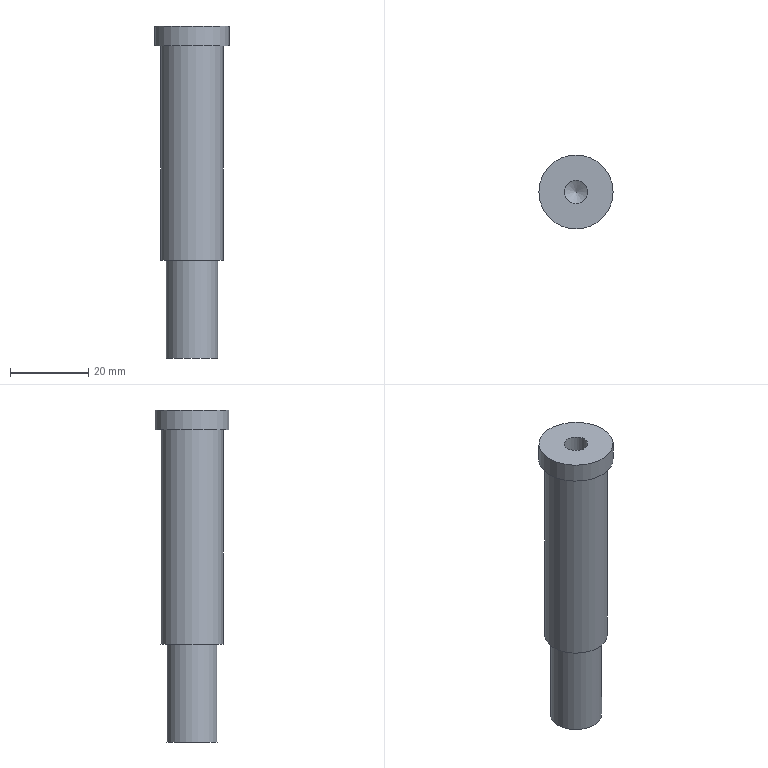Part | NX | features solid 2 | 1 solid | 9 faces | box 19 x 19 x 85 mm | volume 15462 mm3 | cylinder 4 | plane 4 | cone 1 | commonest cylinder face diameters 6 x1 13.1 x1 16 x1 19 x1
STEP:
#1=CARTESIAN_POINT('',(315.095,40.004,20.));
#2=VERTEX_POINT('',#1);
#3=CARTESIAN_POINT('',(307.095,40.004,20.));
#4=DIRECTION('',(0.,0.,1.));
#5=DIRECTION('',(1.,0.,0.));
#6=AXIS2_PLACEMENT_3D('',#3,#4,#5);
#7=CIRCLE('',#6,8.);
#8=EDGE_CURVE('',#2,#2,#7,.T.);
#9=ORIENTED_EDGE('',*,*,#8,.T.);
#10=EDGE_LOOP('',(#9));
#11=FACE_BOUND('',#10,.T.);
#12=CARTESIAN_POINT('',(315.095,40.004,75.));
#13=VERTEX_POINT('',#12);
#14=CARTESIAN_POINT('',(307.095,40.004,75.));
#15=DIRECTION('',(0.,0.,1.));
#16=DIRECTION('',(1.,0.,0.));
#17=AXIS2_PLACEMENT_3D('',#14,#15,#16);
#18=CIRCLE('',#17,8.);
#19=EDGE_CURVE('',#13,#13,#18,.T.);
#20=ORIENTED_EDGE('',*,*,#19,.F.);
#21=EDGE_LOOP('',(#20));
#22=FACE_BOUND('',#21,.T.);
#23=CARTESIAN_POINT('',(307.095,40.004,75.));
#24=DIRECTION('',(0.,0.,-1.));
#25=DIRECTION('',(-1.,0.,0.));
#26=AXIS2_PLACEMENT_3D('',#23,#24,#25);
#27=CYLINDRICAL_SURFACE('',#26,8.);
#28=ADVANCED_FACE('',(#11,#22),#27,.T.);
#29=CARTESIAN_POINT('',(313.645,40.004,20.));
#30=VERTEX_POINT('',#29);
#31=CARTESIAN_POINT('',(307.095,40.004,20.));
#32=DIRECTION('',(0.,0.,1.));
#33=DIRECTION('',(1.,0.,0.));
#34=AXIS2_PLACEMENT_3D('',#31,#32,#33);
#35=CIRCLE('',#34,6.55);
#36=EDGE_CURVE('',#30,#30,#35,.T.);
#37=ORIENTED_EDGE('',*,*,#36,.T.);
#38=EDGE_LOOP('',(#37));
#39=FACE_BOUND('',#38,.T.);
#40=ORIENTED_EDGE('',*,*,#8,.F.);
#41=EDGE_LOOP('',(#40));
#42=FACE_BOUND('',#41,.T.);
#43=CARTESIAN_POINT('',(307.095,40.004,20.));
#44=DIRECTION('',(0.,0.,1.));
#45=DIRECTION('',(1.,0.,0.));
#46=AXIS2_PLACEMENT_3D('',#43,#44,#45);
#47=PLANE('',#46);
#48=ADVANCED_FACE('',(#39,#42),#47,.F.);
#49=CARTESIAN_POINT('',(316.595,40.004,75.));
#50=VERTEX_POINT('',#49);
#51=CARTESIAN_POINT('',(307.095,40.004,75.));
#52=DIRECTION('',(0.,0.,1.));
#53=DIRECTION('',(1.,0.,0.));
#54=AXIS2_PLACEMENT_3D('',#51,#52,#53);
#55=CIRCLE('',#54,9.5);
#56=EDGE_CURVE('',#50,#50,#55,.T.);
#57=ORIENTED_EDGE('',*,*,#56,.F.);
#58=EDGE_LOOP('',(#57));
#59=FACE_BOUND('',#58,.T.);
#60=ORIENTED_EDGE('',*,*,#19,.T.);
#61=EDGE_LOOP('',(#60));
#62=FACE_BOUND('',#61,.T.);
#63=CARTESIAN_POINT('',(307.095,40.004,75.));
#64=DIRECTION('',(0.,0.,1.));
#65=DIRECTION('',(1.,0.,0.));
#66=AXIS2_PLACEMENT_3D('',#63,#64,#65);
#67=PLANE('',#66);
#68=ADVANCED_FACE('',(#59,#62),#67,.F.);
#69=ORIENTED_EDGE('',*,*,#56,.T.);
#70=EDGE_LOOP('',(#69));
#71=FACE_BOUND('',#70,.T.);
#72=CARTESIAN_POINT('',(316.595,40.004,80.));
#73=VERTEX_POINT('',#72);
#74=CARTESIAN_POINT('',(307.095,40.004,80.));
#75=DIRECTION('',(0.,0.,1.));
#76=DIRECTION('',(1.,0.,0.));
#77=AXIS2_PLACEMENT_3D('',#74,#75,#76);
#78=CIRCLE('',#77,9.5);
#79=EDGE_CURVE('',#73,#73,#78,.T.);
#80=ORIENTED_EDGE('',*,*,#79,.F.);
#81=EDGE_LOOP('',(#80));
#82=FACE_BOUND('',#81,.T.);
#83=CARTESIAN_POINT('',(307.095,40.004,70.));
#84=DIRECTION('',(0.,0.,1.));
#85=DIRECTION('',(1.,0.,0.));
#86=AXIS2_PLACEMENT_3D('',#83,#84,#85);
#87=CYLINDRICAL_SURFACE('',#86,9.5);
#88=ADVANCED_FACE('',(#71,#82),#87,.T.);
#89=CARTESIAN_POINT('',(304.095,40.004,80.));
#90=VERTEX_POINT('',#89);
#91=CARTESIAN_POINT('',(307.095,40.004,80.));
#92=DIRECTION('',(0.,0.,-1.));
#93=DIRECTION('',(-1.,0.,0.));
#94=AXIS2_PLACEMENT_3D('',#91,#92,#93);
#95=CIRCLE('',#94,3.);
#96=EDGE_CURVE('',#90,#90,#95,.T.);
#97=ORIENTED_EDGE('',*,*,#96,.T.);
#98=EDGE_LOOP('',(#97));
#99=FACE_BOUND('',#98,.T.);
#100=ORIENTED_EDGE('',*,*,#79,.T.);
#101=EDGE_LOOP('',(#100));
#102=FACE_BOUND('',#101,.T.);
#103=CARTESIAN_POINT('',(307.095,40.004,80.));
#104=DIRECTION('',(0.,0.,1.));
#105=DIRECTION('',(1.,0.,0.));
#106=AXIS2_PLACEMENT_3D('',#103,#104,#105);
#107=PLANE('',#106);
#108=ADVANCED_FACE('',(#99,#102),#107,.T.);
#109=CARTESIAN_POINT('',(313.645,40.004,-5.));
#110=VERTEX_POINT('',#109);
#111=CARTESIAN_POINT('',(307.095,40.004,-5.));
#112=DIRECTION('',(0.,0.,1.));
#113=DIRECTION('',(1.,0.,0.));
#114=AXIS2_PLACEMENT_3D('',#111,#112,#113);
#115=CIRCLE('',#114,6.55);
#116=EDGE_CURVE('',#110,#110,#115,.T.);
#117=ORIENTED_EDGE('',*,*,#116,.T.);
#118=EDGE_LOOP('',(#117));
#119=FACE_BOUND('',#118,.T.);
#120=ORIENTED_EDGE('',*,*,#36,.F.);
#121=EDGE_LOOP('',(#120));
#122=FACE_BOUND('',#121,.T.);
#123=CARTESIAN_POINT('',(307.095,40.004,-5.));
#124=DIRECTION('',(0.,0.,1.));
#125=DIRECTION('',(1.,0.,0.));
#126=AXIS2_PLACEMENT_3D('',#123,#124,#125);
#127=CYLINDRICAL_SURFACE('',#126,6.55);
#128=ADVANCED_FACE('',(#119,#122),#127,.T.);
#129=ORIENTED_EDGE('',*,*,#116,.F.);
#130=EDGE_LOOP('',(#129));
#131=FACE_BOUND('',#130,.T.);
#132=CARTESIAN_POINT('',(307.095,40.004,-5.));
#133=DIRECTION('',(0.,0.,1.));
#134=DIRECTION('',(1.,0.,0.));
#135=AXIS2_PLACEMENT_3D('',#132,#133,#134);
#136=PLANE('',#135);
#137=ADVANCED_FACE('',(#131),#136,.F.);
#138=CARTESIAN_POINT('',(304.095,40.004,67.));
#139=VERTEX_POINT('',#138);
#140=CARTESIAN_POINT('',(307.095,40.004,67.));
#141=DIRECTION('',(0.,0.,-1.));
#142=DIRECTION('',(-1.,0.,0.));
#143=AXIS2_PLACEMENT_3D('',#140,#141,#142);
#144=CIRCLE('',#143,3.);
#145=EDGE_CURVE('',#139,#139,#144,.T.);
#146=ORIENTED_EDGE('',*,*,#145,.F.);
#147=EDGE_LOOP('',(#146));
#148=FACE_BOUND('',#147,.T.);
#149=CARTESIAN_POINT('',(307.095,40.004,65.268));
#150=VERTEX_POINT('',#149);
#151=VERTEX_LOOP('',#150);
#152=FACE_BOUND('',#151,.T.);
#153=CARTESIAN_POINT('',(307.095,40.004,67.));
#154=DIRECTION('',(0.,0.,1.));
#155=DIRECTION('',(1.,0.,0.));
#156=AXIS2_PLACEMENT_3D('',#153,#154,#155);
#157=CONICAL_SURFACE('',#156,3.,1.047);
#158=ADVANCED_FACE('',(#148,#152),#157,.F.);
#159=ORIENTED_EDGE('',*,*,#145,.T.);
#160=EDGE_LOOP('',(#159));
#161=FACE_BOUND('',#160,.T.);
#162=ORIENTED_EDGE('',*,*,#96,.F.);
#163=EDGE_LOOP('',(#162));
#164=FACE_BOUND('',#163,.T.);
#165=CARTESIAN_POINT('',(307.095,40.004,75.));
#166=DIRECTION('',(0.,0.,-1.));
#167=DIRECTION('',(-1.,0.,0.));
#168=AXIS2_PLACEMENT_3D('',#165,#166,#167);
#169=CYLINDRICAL_SURFACE('',#168,3.);
#170=ADVANCED_FACE('',(#161,#164),#169,.F.);
#171=CLOSED_SHELL('',(#28,#48,#68,#88,#108,#128,#137,#158,#170));
#172=MANIFOLD_SOLID_BREP('',#171);
#173=(LENGTH_UNIT()NAMED_UNIT(*)SI_UNIT(.MILLI.,.METRE.));
#174=UNCERTAINTY_MEASURE_WITH_UNIT(LENGTH_MEASURE(0.00001),#173,'','');
#175=(NAMED_UNIT(*)PLANE_ANGLE_UNIT()SI_UNIT($,.RADIAN.));
#176=(NAMED_UNIT(*)SI_UNIT($,.STERADIAN.)SOLID_ANGLE_UNIT());
#177=(GEOMETRIC_REPRESENTATION_CONTEXT(3)GLOBAL_UNCERTAINTY_ASSIGNED_CONTEXT((#174))GLOBAL_UNIT_ASSIGNED_CONTEXT((#173,#175,#176))REPRESENTATION_CONTEXT('',''));
#178=ADVANCED_BREP_SHAPE_REPRESENTATION('',(#172),#177);